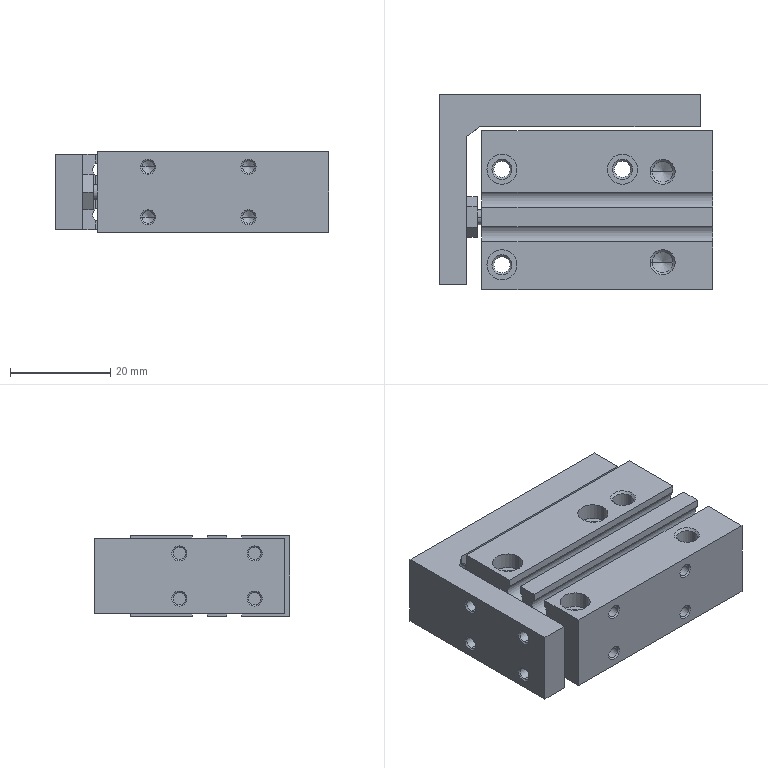Part | STEP file | Compact pneumatic slide MXH6-15Z | 2 solids | 206 faces | box 54.5 x 39 x 16 mm | volume 25990 mm3 | cone 86 | cylinder 76 | plane 44 | commonest cylinder face diameters 2.459 x32 6 x16 4.134 x12 3.242 x6 4.2 x6 3 x2